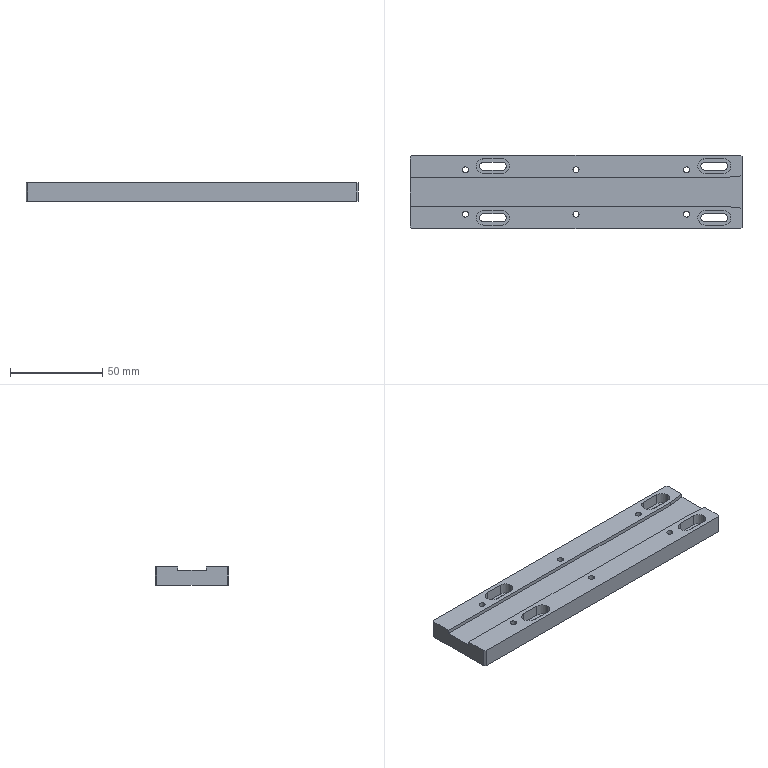Part | STEP file | PN_0040 linear vibrating groove | 1 solid | 72 faces | box 180 x 40 x 10 mm | volume 61766 mm3 | cylinder 36 | plane 36 | commonest cylinder face diameters 3.3 x12 4.5 x12 8 x12